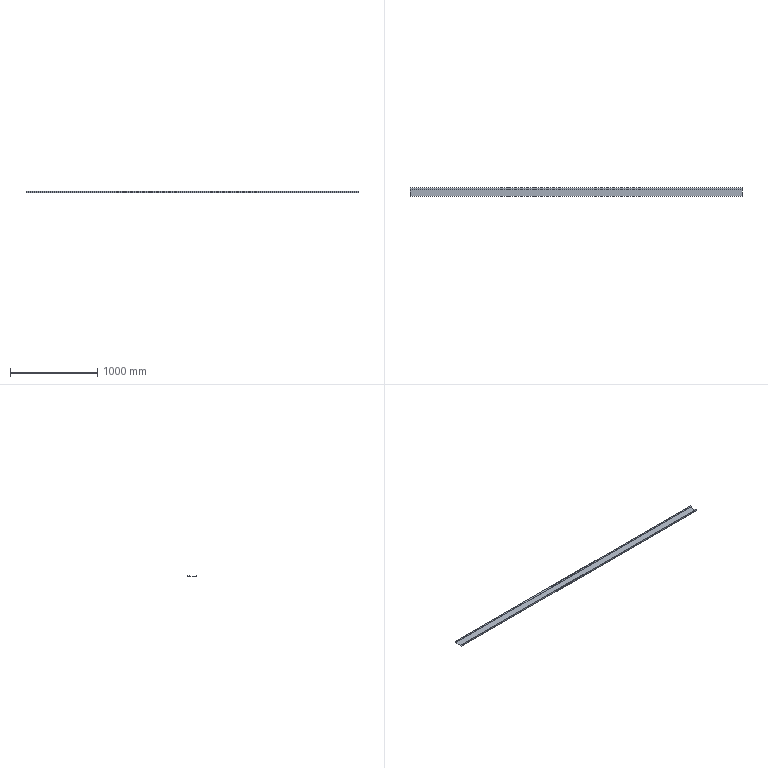Part | STEP file | 粉仓踢脚Plate 2 | 1 solid | 18 faces | box 3814 x 100 x 20 mm | volume 876724 mm3 | plane 12 | cylinder 6 | commonest cylinder face diameters 2 x3 5 x3
STEP:
#1=CARTESIAN_POINT('',(0.,0.,0.));
#2=DIRECTION('',(0.,0.,1.));
#3=DIRECTION('',(1.,0.,0.));
#4=AXIS2_PLACEMENT_3D('',#1,#2,#3);
#5=CARTESIAN_POINT('',(-1907.,1.5,2.5));
#6=VERTEX_POINT('',#5);
#7=CARTESIAN_POINT('',(-1907.,1.5,20.));
#8=VERTEX_POINT('',#7);
#9=CARTESIAN_POINT('',(-1907.,1.5,2.5));
#10=DIRECTION('',(0.,0.,1.));
#11=VECTOR('',#10,1.);
#12=LINE('',#9,#11);
#13=CARTESIAN_POINT('',(1907.,1.5,2.5));
#14=DIRECTION('',(0.,-1.,0.));
#15=DIRECTION('',(0.,0.,-1.));
#16=AXIS2_PLACEMENT_3D('',#13,#14,#15);
#17=PLANE('',#16);
#18=CARTESIAN_POINT('',(0.,-3814.));
#19=DIRECTION('',(-1.,0.));
#20=VECTOR('',#19,1.);
#21=LINE('',#18,#20);
#22=(GEOMETRIC_REPRESENTATION_CONTEXT(2)PARAMETRIC_REPRESENTATION_CONTEXT()REPRESENTATION_CONTEXT('',''));
#23=DEFINITIONAL_REPRESENTATION('',(#21),#22);
#24=PCURVE('',#17,#23);
#25=CARTESIAN_POINT('',(-1907.,2.5,2.5));
#26=DIRECTION('',(-1.,0.,0.));
#27=DIRECTION('',(0.,0.,1.));
#28=AXIS2_PLACEMENT_3D('',#25,#26,#27);
#29=PLANE('',#28);
#30=CARTESIAN_POINT('',(0.,-1.));
#31=DIRECTION('',(1.,0.));
#32=VECTOR('',#31,1.);
#33=LINE('',#30,#32);
#34=(GEOMETRIC_REPRESENTATION_CONTEXT(2)PARAMETRIC_REPRESENTATION_CONTEXT()REPRESENTATION_CONTEXT('',''));
#35=DEFINITIONAL_REPRESENTATION('',(#33),#34);
#36=PCURVE('',#29,#35);
#37=SURFACE_CURVE('',#12,(#24,#36),.PCURVE_S1.);
#38=EDGE_CURVE('',#6,#8,#37,.T.);
#39=ORIENTED_EDGE('',*,*,#38,.T.);
#40=CARTESIAN_POINT('',(1907.,1.5,20.));
#41=VERTEX_POINT('',#40);
#42=CARTESIAN_POINT('',(1907.,1.5,20.));
#43=DIRECTION('',(-1.,0.,0.));
#44=VECTOR('',#43,1.);
#45=LINE('',#42,#44);
#46=CARTESIAN_POINT('',(-17.5,0.));
#47=DIRECTION('',(0.,-1.));
#48=VECTOR('',#47,1.);
#49=LINE('',#46,#48);
#50=(GEOMETRIC_REPRESENTATION_CONTEXT(2)PARAMETRIC_REPRESENTATION_CONTEXT()REPRESENTATION_CONTEXT('',''));
#51=DEFINITIONAL_REPRESENTATION('',(#49),#50);
#52=PCURVE('',#17,#51);
#53=CARTESIAN_POINT('',(1907.,0.,20.));
#54=DIRECTION('',(0.,0.,1.));
#55=DIRECTION('',(1.,0.,0.));
#56=AXIS2_PLACEMENT_3D('',#53,#54,#55);
#57=PLANE('',#56);
#58=CARTESIAN_POINT('',(0.,1.5));
#59=DIRECTION('',(-1.,0.));
#60=VECTOR('',#59,1.);
#61=LINE('',#58,#60);
#62=(GEOMETRIC_REPRESENTATION_CONTEXT(2)PARAMETRIC_REPRESENTATION_CONTEXT()REPRESENTATION_CONTEXT('',''));
#63=DEFINITIONAL_REPRESENTATION('',(#61),#62);
#64=PCURVE('',#57,#63);
#65=SURFACE_CURVE('',#45,(#52,#64),.PCURVE_S1.);
#66=EDGE_CURVE('',#41,#8,#65,.T.);
#67=ORIENTED_EDGE('',*,*,#66,.F.);
#68=CARTESIAN_POINT('',(1907.,1.5,2.5));
#69=VERTEX_POINT('',#68);
#70=CARTESIAN_POINT('',(1907.,1.5,2.5));
#71=DIRECTION('',(0.,0.,1.));
#72=VECTOR('',#71,1.);
#73=LINE('',#70,#72);
#74=CARTESIAN_POINT('',(0.,0.));
#75=DIRECTION('',(-1.,0.));
#76=VECTOR('',#75,1.);
#77=LINE('',#74,#76);
#78=(GEOMETRIC_REPRESENTATION_CONTEXT(2)PARAMETRIC_REPRESENTATION_CONTEXT()REPRESENTATION_CONTEXT('',''));
#79=DEFINITIONAL_REPRESENTATION('',(#77),#78);
#80=PCURVE('',#17,#79);
#81=CARTESIAN_POINT('',(1907.,2.5,2.5));
#82=DIRECTION('',(-1.,0.,0.));
#83=DIRECTION('',(0.,0.,1.));
#84=AXIS2_PLACEMENT_3D('',#81,#82,#83);
#85=PLANE('',#84);
#86=CARTESIAN_POINT('',(0.,-1.));
#87=DIRECTION('',(1.,0.));
#88=VECTOR('',#87,1.);
#89=LINE('',#86,#88);
#90=(GEOMETRIC_REPRESENTATION_CONTEXT(2)PARAMETRIC_REPRESENTATION_CONTEXT()REPRESENTATION_CONTEXT('',''));
#91=DEFINITIONAL_REPRESENTATION('',(#89),#90);
#92=PCURVE('',#85,#91);
#93=SURFACE_CURVE('',#73,(#80,#92),.PCURVE_S1.);
#94=EDGE_CURVE('',#69,#41,#93,.T.);
#95=ORIENTED_EDGE('',*,*,#94,.F.);
#96=CARTESIAN_POINT('',(1907.,1.5,2.5));
#97=DIRECTION('',(-1.,0.,0.));
#98=VECTOR('',#97,1.);
#99=LINE('',#96,#98);
#100=CARTESIAN_POINT('',(0.,0.));
#101=DIRECTION('',(0.,-1.));
#102=VECTOR('',#101,1.);
#103=LINE('',#100,#102);
#104=(GEOMETRIC_REPRESENTATION_CONTEXT(2)PARAMETRIC_REPRESENTATION_CONTEXT()REPRESENTATION_CONTEXT('',''));
#105=DEFINITIONAL_REPRESENTATION('',(#103),#104);
#106=PCURVE('',#17,#105);
#107=CARTESIAN_POINT('',(1907.,2.5,2.5));
#108=DIRECTION('',(-1.,0.,0.));
#109=DIRECTION('',(0.,0.,1.));
#110=AXIS2_PLACEMENT_3D('',#107,#108,#109);
#111=CYLINDRICAL_SURFACE('',#110,1.);
#112=CARTESIAN_POINT('',(4.712,0.));
#113=DIRECTION('',(0.,1.));
#114=VECTOR('',#113,1.);
#115=LINE('',#112,#114);
#116=(GEOMETRIC_REPRESENTATION_CONTEXT(2)PARAMETRIC_REPRESENTATION_CONTEXT()REPRESENTATION_CONTEXT('',''));
#117=DEFINITIONAL_REPRESENTATION('',(#115),#116);
#118=PCURVE('',#111,#117);
#119=SURFACE_CURVE('',#99,(#106,#118),.PCURVE_S1.);
#120=EDGE_CURVE('',#69,#6,#119,.T.);
#121=ORIENTED_EDGE('',*,*,#120,.T.);
#122=EDGE_LOOP('',(#39,#67,#95,#121));
#123=FACE_BOUND('',#122,.T.);
#124=ADVANCED_FACE('',(#123),#17,.F.);
#125=CARTESIAN_POINT('',(-1907.,0.,20.));
#126=VERTEX_POINT('',#125);
#127=CARTESIAN_POINT('',(-1907.,0.,20.));
#128=DIRECTION('',(0.,1.,0.));
#129=VECTOR('',#128,1.);
#130=LINE('',#127,#129);
#131=CARTESIAN_POINT('',(-3814.,0.));
#132=DIRECTION('',(0.,1.));
#133=VECTOR('',#132,1.);
#134=LINE('',#131,#133);
#135=(GEOMETRIC_REPRESENTATION_CONTEXT(2)PARAMETRIC_REPRESENTATION_CONTEXT()REPRESENTATION_CONTEXT('',''));
#136=DEFINITIONAL_REPRESENTATION('',(#134),#135);
#137=PCURVE('',#57,#136);
#138=CARTESIAN_POINT('',(17.5,-2.5));
#139=DIRECTION('',(0.,1.));
#140=VECTOR('',#139,1.);
#141=LINE('',#138,#140);
#142=(GEOMETRIC_REPRESENTATION_CONTEXT(2)PARAMETRIC_REPRESENTATION_CONTEXT()REPRESENTATION_CONTEXT('',''));
#143=DEFINITIONAL_REPRESENTATION('',(#141),#142);
#144=PCURVE('',#29,#143);
#145=SURFACE_CURVE('',#130,(#137,#144),.PCURVE_S1.);
#146=EDGE_CURVE('',#126,#8,#145,.T.);
#147=ORIENTED_EDGE('',*,*,#146,.F.);
#148=CARTESIAN_POINT('',(1907.,0.,20.));
#149=VERTEX_POINT('',#148);
#150=CARTESIAN_POINT('',(1907.,0.,20.));
#151=DIRECTION('',(-1.,0.,0.));
#152=VECTOR('',#151,1.);
#153=LINE('',#150,#152);
#154=CARTESIAN_POINT('',(0.,0.));
#155=DIRECTION('',(-1.,0.));
#156=VECTOR('',#155,1.);
#157=LINE('',#154,#156);
#158=(GEOMETRIC_REPRESENTATION_CONTEXT(2)PARAMETRIC_REPRESENTATION_CONTEXT()REPRESENTATION_CONTEXT('',''));
#159=DEFINITIONAL_REPRESENTATION('',(#157),#158);
#160=PCURVE('',#57,#159);
#161=CARTESIAN_POINT('',(1907.,0.,2.5));
#162=DIRECTION('',(0.,-1.,0.));
#163=DIRECTION('',(0.,0.,-1.));
#164=AXIS2_PLACEMENT_3D('',#161,#162,#163);
#165=PLANE('',#164);
#166=CARTESIAN_POINT('',(-17.5,0.));
#167=DIRECTION('',(0.,-1.));
#168=VECTOR('',#167,1.);
#169=LINE('',#166,#168);
#170=(GEOMETRIC_REPRESENTATION_CONTEXT(2)PARAMETRIC_REPRESENTATION_CONTEXT()REPRESENTATION_CONTEXT('',''));
#171=DEFINITIONAL_REPRESENTATION('',(#169),#170);
#172=PCURVE('',#165,#171);
#173=SURFACE_CURVE('',#153,(#160,#172),.PCURVE_S1.);
#174=EDGE_CURVE('',#149,#126,#173,.T.);
#175=ORIENTED_EDGE('',*,*,#174,.F.);
#176=CARTESIAN_POINT('',(1907.,0.,20.));
#177=DIRECTION('',(0.,1.,0.));
#178=VECTOR('',#177,1.);
#179=LINE('',#176,#178);
#180=CARTESIAN_POINT('',(0.,0.));
#181=DIRECTION('',(0.,1.));
#182=VECTOR('',#181,1.);
#183=LINE('',#180,#182);
#184=(GEOMETRIC_REPRESENTATION_CONTEXT(2)PARAMETRIC_REPRESENTATION_CONTEXT()REPRESENTATION_CONTEXT('',''));
#185=DEFINITIONAL_REPRESENTATION('',(#183),#184);
#186=PCURVE('',#57,#185);
#187=CARTESIAN_POINT('',(17.5,-2.5));
#188=DIRECTION('',(0.,1.));
#189=VECTOR('',#188,1.);
#190=LINE('',#187,#189);
#191=(GEOMETRIC_REPRESENTATION_CONTEXT(2)PARAMETRIC_REPRESENTATION_CONTEXT()REPRESENTATION_CONTEXT('',''));
#192=DEFINITIONAL_REPRESENTATION('',(#190),#191);
#193=PCURVE('',#85,#192);
#194=SURFACE_CURVE('',#179,(#186,#193),.PCURVE_S1.);
#195=EDGE_CURVE('',#149,#41,#194,.T.);
#196=ORIENTED_EDGE('',*,*,#195,.T.);
#197=ORIENTED_EDGE('',*,*,#66,.T.);
#198=EDGE_LOOP('',(#147,#175,#196,#197));
#199=FACE_BOUND('',#198,.T.);
#200=ADVANCED_FACE('',(#199),#57,.T.);
#201=CARTESIAN_POINT('',(-1907.,0.,2.5));
#202=VERTEX_POINT('',#201);
#203=CARTESIAN_POINT('',(-1907.,0.,2.5));
#204=DIRECTION('',(0.,0.,1.));
#205=VECTOR('',#204,1.);
#206=LINE('',#203,#205);
#207=CARTESIAN_POINT('',(0.,-3814.));
#208=DIRECTION('',(-1.,0.));
#209=VECTOR('',#208,1.);
#210=LINE('',#207,#209);
#211=(GEOMETRIC_REPRESENTATION_CONTEXT(2)PARAMETRIC_REPRESENTATION_CONTEXT()REPRESENTATION_CONTEXT('',''));
#212=DEFINITIONAL_REPRESENTATION('',(#210),#211);
#213=PCURVE('',#165,#212);
#214=CARTESIAN_POINT('',(0.,-2.5));
#215=DIRECTION('',(1.,0.));
#216=VECTOR('',#215,1.);
#217=LINE('',#214,#216);
#218=(GEOMETRIC_REPRESENTATION_CONTEXT(2)PARAMETRIC_REPRESENTATION_CONTEXT()REPRESENTATION_CONTEXT('',''));
#219=DEFINITIONAL_REPRESENTATION('',(#217),#218);
#220=PCURVE('',#29,#219);
#221=SURFACE_CURVE('',#206,(#213,#220),.PCURVE_S1.);
#222=EDGE_CURVE('',#202,#126,#221,.T.);
#223=ORIENTED_EDGE('',*,*,#222,.F.);
#224=CARTESIAN_POINT('',(1907.,0.,2.5));
#225=VERTEX_POINT('',#224);
#226=CARTESIAN_POINT('',(1907.,0.,2.5));
#227=DIRECTION('',(-1.,0.,0.));
#228=VECTOR('',#227,1.);
#229=LINE('',#226,#228);
#230=CARTESIAN_POINT('',(0.,0.));
#231=DIRECTION('',(0.,-1.));
#232=VECTOR('',#231,1.);
#233=LINE('',#230,#232);
#234=(GEOMETRIC_REPRESENTATION_CONTEXT(2)PARAMETRIC_REPRESENTATION_CONTEXT()REPRESENTATION_CONTEXT('',''));
#235=DEFINITIONAL_REPRESENTATION('',(#233),#234);
#236=PCURVE('',#165,#235);
#237=CARTESIAN_POINT('',(1907.,2.5,2.5));
#238=DIRECTION('',(-1.,0.,0.));
#239=DIRECTION('',(0.,0.,1.));
#240=AXIS2_PLACEMENT_3D('',#237,#238,#239);
#241=CYLINDRICAL_SURFACE('',#240,2.5);
#242=CARTESIAN_POINT('',(4.712,0.));
#243=DIRECTION('',(0.,1.));
#244=VECTOR('',#243,1.);
#245=LINE('',#242,#244);
#246=(GEOMETRIC_REPRESENTATION_CONTEXT(2)PARAMETRIC_REPRESENTATION_CONTEXT()REPRESENTATION_CONTEXT('',''));
#247=DEFINITIONAL_REPRESENTATION('',(#245),#246);
#248=PCURVE('',#241,#247);
#249=SURFACE_CURVE('',#229,(#236,#248),.PCURVE_S1.);
#250=EDGE_CURVE('',#225,#202,#249,.T.);
#251=ORIENTED_EDGE('',*,*,#250,.F.);
#252=CARTESIAN_POINT('',(1907.,0.,2.5));
#253=DIRECTION('',(0.,0.,1.));
#254=VECTOR('',#253,1.);
#255=LINE('',#252,#254);
#256=CARTESIAN_POINT('',(0.,0.));
#257=DIRECTION('',(-1.,0.));
#258=VECTOR('',#257,1.);
#259=LINE('',#256,#258);
#260=(GEOMETRIC_REPRESENTATION_CONTEXT(2)PARAMETRIC_REPRESENTATION_CONTEXT()REPRESENTATION_CONTEXT('',''));
#261=DEFINITIONAL_REPRESENTATION('',(#259),#260);
#262=PCURVE('',#165,#261);
#263=CARTESIAN_POINT('',(0.,-2.5));
#264=DIRECTION('',(1.,0.));
#265=VECTOR('',#264,1.);
#266=LINE('',#263,#265);
#267=(GEOMETRIC_REPRESENTATION_CONTEXT(2)PARAMETRIC_REPRESENTATION_CONTEXT()REPRESENTATION_CONTEXT('',''));
#268=DEFINITIONAL_REPRESENTATION('',(#266),#267);
#269=PCURVE('',#85,#268);
#270=SURFACE_CURVE('',#255,(#262,#269),.PCURVE_S1.);
#271=EDGE_CURVE('',#225,#149,#270,.T.);
#272=ORIENTED_EDGE('',*,*,#271,.T.);
#273=ORIENTED_EDGE('',*,*,#174,.T.);
#274=EDGE_LOOP('',(#223,#251,#272,#273));
#275=FACE_BOUND('',#274,.T.);
#276=ADVANCED_FACE('',(#275),#165,.T.);
#277=CARTESIAN_POINT('',(-1907.,2.5,0.));
#278=VERTEX_POINT('',#277);
#279=CARTESIAN_POINT('',(-1907.,2.5,2.5));
#280=DIRECTION('',(-1.,0.,0.));
#281=DIRECTION('',(0.,0.,1.));
#282=AXIS2_PLACEMENT_3D('',#279,#280,#281);
#283=CIRCLE('',#282,2.5);
#284=CARTESIAN_POINT('',(0.,3814.));
#285=DIRECTION('',(1.,0.));
#286=VECTOR('',#285,1.);
#287=LINE('',#284,#286);
#288=(GEOMETRIC_REPRESENTATION_CONTEXT(2)PARAMETRIC_REPRESENTATION_CONTEXT()REPRESENTATION_CONTEXT('',''));
#289=DEFINITIONAL_REPRESENTATION('',(#287),#288);
#290=PCURVE('',#241,#289);
#291=CARTESIAN_POINT('',(0.,0.));
#292=DIRECTION('',(1.,0.));
#293=AXIS2_PLACEMENT_2D('',#291,#292);
#294=CIRCLE('',#293,2.5);
#295=(GEOMETRIC_REPRESENTATION_CONTEXT(2)PARAMETRIC_REPRESENTATION_CONTEXT()REPRESENTATION_CONTEXT('',''));
#296=DEFINITIONAL_REPRESENTATION('',(#294),#295);
#297=PCURVE('',#29,#296);
#298=SURFACE_CURVE('',#283,(#290,#297),.PCURVE_S1.);
#299=EDGE_CURVE('',#278,#202,#298,.T.);
#300=ORIENTED_EDGE('',*,*,#299,.F.);
#301=CARTESIAN_POINT('',(1907.,2.5,0.));
#302=VERTEX_POINT('',#301);
#303=CARTESIAN_POINT('',(1907.,2.5,0.));
#304=DIRECTION('',(-1.,0.,0.));
#305=VECTOR('',#304,1.);
#306=LINE('',#303,#305);
#307=CARTESIAN_POINT('',(3.142,0.));
#308=DIRECTION('',(0.,1.));
#309=VECTOR('',#308,1.);
#310=LINE('',#307,#309);
#311=(GEOMETRIC_REPRESENTATION_CONTEXT(2)PARAMETRIC_REPRESENTATION_CONTEXT()REPRESENTATION_CONTEXT('',''));
#312=DEFINITIONAL_REPRESENTATION('',(#310),#311);
#313=PCURVE('',#241,#312);
#314=CARTESIAN_POINT('',(1907.,2.5,0.));
#315=DIRECTION('',(0.,0.,-1.));
#316=DIRECTION('',(-1.,0.,0.));
#317=AXIS2_PLACEMENT_3D('',#314,#315,#316);
#318=PLANE('',#317);
#319=CARTESIAN_POINT('',(0.,0.));
#320=DIRECTION('',(1.,0.));
#321=VECTOR('',#320,1.);
#322=LINE('',#319,#321);
#323=(GEOMETRIC_REPRESENTATION_CONTEXT(2)PARAMETRIC_REPRESENTATION_CONTEXT()REPRESENTATION_CONTEXT('',''));
#324=DEFINITIONAL_REPRESENTATION('',(#322),#323);
#325=PCURVE('',#318,#324);
#326=SURFACE_CURVE('',#306,(#313,#325),.PCURVE_S1.);
#327=EDGE_CURVE('',#302,#278,#326,.T.);
#328=ORIENTED_EDGE('',*,*,#327,.F.);
#329=CARTESIAN_POINT('',(1907.,2.5,2.5));
#330=DIRECTION('',(-1.,0.,0.));
#331=DIRECTION('',(0.,0.,1.));
#332=AXIS2_PLACEMENT_3D('',#329,#330,#331);
#333=CIRCLE('',#332,2.5);
#334=CARTESIAN_POINT('',(0.,0.));
#335=DIRECTION('',(1.,0.));
#336=VECTOR('',#335,1.);
#337=LINE('',#334,#336);
#338=(GEOMETRIC_REPRESENTATION_CONTEXT(2)PARAMETRIC_REPRESENTATION_CONTEXT()REPRESENTATION_CONTEXT('',''));
#339=DEFINITIONAL_REPRESENTATION('',(#337),#338);
#340=PCURVE('',#241,#339);
#341=CARTESIAN_POINT('',(0.,0.));
#342=DIRECTION('',(1.,0.));
#343=AXIS2_PLACEMENT_2D('',#341,#342);
#344=CIRCLE('',#343,2.5);
#345=(GEOMETRIC_REPRESENTATION_CONTEXT(2)PARAMETRIC_REPRESENTATION_CONTEXT()REPRESENTATION_CONTEXT('',''));
#346=DEFINITIONAL_REPRESENTATION('',(#344),#345);
#347=PCURVE('',#85,#346);
#348=SURFACE_CURVE('',#333,(#340,#347),.PCURVE_S1.);
#349=EDGE_CURVE('',#302,#225,#348,.T.);
#350=ORIENTED_EDGE('',*,*,#349,.T.);
#351=ORIENTED_EDGE('',*,*,#250,.T.);
#352=EDGE_LOOP('',(#300,#328,#350,#351));
#353=FACE_BOUND('',#352,.T.);
#354=ADVANCED_FACE('',(#353),#241,.T.);
#355=CARTESIAN_POINT('',(-1907.,97.5,0.));
#356=VERTEX_POINT('',#355);
#357=CARTESIAN_POINT('',(-1907.,2.5,0.));
#358=DIRECTION('',(0.,-1.,0.));
#359=VECTOR('',#358,1.);
#360=LINE('',#357,#359);
#361=CARTESIAN_POINT('',(3814.,0.));
#362=DIRECTION('',(0.,-1.));
#363=VECTOR('',#362,1.);
#364=LINE('',#361,#363);
#365=(GEOMETRIC_REPRESENTATION_CONTEXT(2)PARAMETRIC_REPRESENTATION_CONTEXT()REPRESENTATION_CONTEXT('',''));
#366=DEFINITIONAL_REPRESENTATION('',(#364),#365);
#367=PCURVE('',#318,#366);
#368=CARTESIAN_POINT('',(-2.5,0.));
#369=DIRECTION('',(0.,-1.));
#370=VECTOR('',#369,1.);
#371=LINE('',#368,#370);
#372=(GEOMETRIC_REPRESENTATION_CONTEXT(2)PARAMETRIC_REPRESENTATION_CONTEXT()REPRESENTATION_CONTEXT('',''));
#373=DEFINITIONAL_REPRESENTATION('',(#371),#372);
#374=PCURVE('',#29,#373);
#375=SURFACE_CURVE('',#360,(#367,#374),.PCURVE_S1.);
#376=EDGE_CURVE('',#356,#278,#375,.T.);
#377=ORIENTED_EDGE('',*,*,#376,.F.);
#378=CARTESIAN_POINT('',(1907.,97.5,0.));
#379=VERTEX_POINT('',#378);
#380=CARTESIAN_POINT('',(1907.,97.5,0.));
#381=DIRECTION('',(-1.,0.,0.));
#382=VECTOR('',#381,1.);
#383=LINE('',#380,#382);
#384=CARTESIAN_POINT('',(0.,95.));
#385=DIRECTION('',(1.,0.));
#386=VECTOR('',#385,1.);
#387=LINE('',#384,#386);
#388=(GEOMETRIC_REPRESENTATION_CONTEXT(2)PARAMETRIC_REPRESENTATION_CONTEXT()REPRESENTATION_CONTEXT('',''));
#389=DEFINITIONAL_REPRESENTATION('',(#387),#388);
#390=PCURVE('',#318,#389);
#391=CARTESIAN_POINT('',(1907.,97.5,2.5));
#392=DIRECTION('',(-1.,0.,0.));
#393=DIRECTION('',(0.,0.,1.));
#394=AXIS2_PLACEMENT_3D('',#391,#392,#393);
#395=CYLINDRICAL_SURFACE('',#394,2.5);
#396=CARTESIAN_POINT('',(3.142,0.));
#397=DIRECTION('',(0.,1.));
#398=VECTOR('',#397,1.);
#399=LINE('',#396,#398);
#400=(GEOMETRIC_REPRESENTATION_CONTEXT(2)PARAMETRIC_REPRESENTATION_CONTEXT()REPRESENTATION_CONTEXT('',''));
#401=DEFINITIONAL_REPRESENTATION('',(#399),#400);
#402=PCURVE('',#395,#401);
#403=SURFACE_CURVE('',#383,(#390,#402),.PCURVE_S1.);
#404=EDGE_CURVE('',#379,#356,#403,.T.);
#405=ORIENTED_EDGE('',*,*,#404,.F.);
#406=CARTESIAN_POINT('',(1907.,2.5,0.));
#407=DIRECTION('',(0.,-1.,0.));
#408=VECTOR('',#407,1.);
#409=LINE('',#406,#408);
#410=CARTESIAN_POINT('',(0.,0.));
#411=DIRECTION('',(0.,-1.));
#412=VECTOR('',#411,1.);
#413=LINE('',#410,#412);
#414=(GEOMETRIC_REPRESENTATION_CONTEXT(2)PARAMETRIC_REPRESENTATION_CONTEXT()REPRESENTATION_CONTEXT('',''));
#415=DEFINITIONAL_REPRESENTATION('',(#413),#414);
#416=PCURVE('',#318,#415);
#417=CARTESIAN_POINT('',(-2.5,0.));
#418=DIRECTION('',(0.,-1.));
#419=VECTOR('',#418,1.);
#420=LINE('',#417,#419);
#421=(GEOMETRIC_REPRESENTATION_CONTEXT(2)PARAMETRIC_REPRESENTATION_CONTEXT()REPRESENTATION_CONTEXT('',''));
#422=DEFINITIONAL_REPRESENTATION('',(#420),#421);
#423=PCURVE('',#85,#422);
#424=SURFACE_CURVE('',#409,(#416,#423),.PCURVE_S1.);
#425=EDGE_CURVE('',#379,#302,#424,.T.);
#426=ORIENTED_EDGE('',*,*,#425,.T.);
#427=ORIENTED_EDGE('',*,*,#327,.T.);
#428=EDGE_LOOP('',(#377,#405,#426,#427));
#429=FACE_BOUND('',#428,.T.);
#430=ADVANCED_FACE('',(#429),#318,.T.);
#431=CARTESIAN_POINT('',(-1907.,100.,2.5));
#432=VERTEX_POINT('',#431);
#433=CARTESIAN_POINT('',(-1907.,97.5,2.5));
#434=DIRECTION('',(-1.,0.,0.));
#435=DIRECTION('',(0.,0.,-1.));
#436=AXIS2_PLACEMENT_3D('',#433,#434,#435);
#437=CIRCLE('',#436,2.5);
#438=CARTESIAN_POINT('',(-3.142,3814.));
#439=DIRECTION('',(1.,0.));
#440=VECTOR('',#439,1.);
#441=LINE('',#438,#440);
#442=(GEOMETRIC_REPRESENTATION_CONTEXT(2)PARAMETRIC_REPRESENTATION_CONTEXT()REPRESENTATION_CONTEXT('',''));
#443=DEFINITIONAL_REPRESENTATION('',(#441),#442);
#444=PCURVE('',#395,#443);
#445=CARTESIAN_POINT('',(0.,95.));
#446=DIRECTION('',(-1.,0.));
#447=AXIS2_PLACEMENT_2D('',#445,#446);
#448=CIRCLE('',#447,2.5);
#449=(GEOMETRIC_REPRESENTATION_CONTEXT(2)PARAMETRIC_REPRESENTATION_CONTEXT()REPRESENTATION_CONTEXT('',''));
#450=DEFINITIONAL_REPRESENTATION('',(#448),#449);
#451=PCURVE('',#29,#450);
#452=SURFACE_CURVE('',#437,(#444,#451),.PCURVE_S1.);
#453=EDGE_CURVE('',#432,#356,#452,.T.);
#454=ORIENTED_EDGE('',*,*,#453,.F.);
#455=CARTESIAN_POINT('',(1907.,100.,2.5));
#456=VERTEX_POINT('',#455);
#457=CARTESIAN_POINT('',(1907.,100.,2.5));
#458=DIRECTION('',(-1.,0.,0.));
#459=VECTOR('',#458,1.);
#460=LINE('',#457,#459);
#461=CARTESIAN_POINT('',(1.571,0.));
#462=DIRECTION('',(0.,1.));
#463=VECTOR('',#462,1.);
#464=LINE('',#461,#463);
#465=(GEOMETRIC_REPRESENTATION_CONTEXT(2)PARAMETRIC_REPRESENTATION_CONTEXT()REPRESENTATION_CONTEXT('',''));
#466=DEFINITIONAL_REPRESENTATION('',(#464),#465);
#467=PCURVE('',#395,#466);
#468=CARTESIAN_POINT('',(1907.,100.,2.5));
#469=DIRECTION('',(0.,1.,0.));
#470=DIRECTION('',(0.,0.,1.));
#471=AXIS2_PLACEMENT_3D('',#468,#469,#470);
#472=PLANE('',#471);
#473=CARTESIAN_POINT('',(0.,0.));
#474=DIRECTION('',(0.,-1.));
#475=VECTOR('',#474,1.);
#476=LINE('',#473,#475);
#477=(GEOMETRIC_REPRESENTATION_CONTEXT(2)PARAMETRIC_REPRESENTATION_CONTEXT()REPRESENTATION_CONTEXT('',''));
#478=DEFINITIONAL_REPRESENTATION('',(#476),#477);
#479=PCURVE('',#472,#478);
#480=SURFACE_CURVE('',#460,(#467,#479),.PCURVE_S1.);
#481=EDGE_CURVE('',#456,#432,#480,.T.);
#482=ORIENTED_EDGE('',*,*,#481,.F.);
#483=CARTESIAN_POINT('',(1907.,97.5,2.5));
#484=DIRECTION('',(-1.,0.,0.));
#485=DIRECTION('',(0.,0.,-1.));
#486=AXIS2_PLACEMENT_3D('',#483,#484,#485);
#487=CIRCLE('',#486,2.5);
#488=CARTESIAN_POINT('',(-3.142,0.));
#489=DIRECTION('',(1.,0.));
#490=VECTOR('',#489,1.);
#491=LINE('',#488,#490);
#492=(GEOMETRIC_REPRESENTATION_CONTEXT(2)PARAMETRIC_REPRESENTATION_CONTEXT()REPRESENTATION_CONTEXT('',''));
#493=DEFINITIONAL_REPRESENTATION('',(#491),#492);
#494=PCURVE('',#395,#493);
#495=CARTESIAN_POINT('',(0.,95.));
#496=DIRECTION('',(-1.,0.));
#497=AXIS2_PLACEMENT_2D('',#495,#496);
#498=CIRCLE('',#497,2.5);
#499=(GEOMETRIC_REPRESENTATION_CONTEXT(2)PARAMETRIC_REPRESENTATION_CONTEXT()REPRESENTATION_CONTEXT('',''));
#500=DEFINITIONAL_REPRESENTATION('',(#498),#499);
#501=PCURVE('',#85,#500);
#502=SURFACE_CURVE('',#487,(#494,#501),.PCURVE_S1.);
#503=EDGE_CURVE('',#456,#379,#502,.T.);
#504=ORIENTED_EDGE('',*,*,#503,.T.);
#505=ORIENTED_EDGE('',*,*,#404,.T.);
#506=EDGE_LOOP('',(#454,#482,#504,#505));
#507=FACE_BOUND('',#506,.T.);
#508=ADVANCED_FACE('',(#507),#395,.T.);
#509=CARTESIAN_POINT('',(-1907.,100.,17.5));
#510=VERTEX_POINT('',#509);
#511=CARTESIAN_POINT('',(-1907.,100.,2.5));
#512=DIRECTION('',(0.,0.,-1.));
#513=VECTOR('',#512,1.);
#514=LINE('',#511,#513);
#515=CARTESIAN_POINT('',(0.,-3814.));
#516=DIRECTION('',(-1.,0.));
#517=VECTOR('',#516,1.);
#518=LINE('',#515,#517);
#519=(GEOMETRIC_REPRESENTATION_CONTEXT(2)PARAMETRIC_REPRESENTATION_CONTEXT()REPRESENTATION_CONTEXT('',''));
#520=DEFINITIONAL_REPRESENTATION('',(#518),#519);
#521=PCURVE('',#472,#520);
#522=CARTESIAN_POINT('',(0.,97.5));
#523=DIRECTION('',(-1.,0.));
#524=VECTOR('',#523,1.);
#525=LINE('',#522,#524);
#526=(GEOMETRIC_REPRESENTATION_CONTEXT(2)PARAMETRIC_REPRESENTATION_CONTEXT()REPRESENTATION_CONTEXT('',''));
#527=DEFINITIONAL_REPRESENTATION('',(#525),#526);
#528=PCURVE('',#29,#527);
#529=SURFACE_CURVE('',#514,(#521,#528),.PCURVE_S1.);
#530=EDGE_CURVE('',#510,#432,#529,.T.);
#531=ORIENTED_EDGE('',*,*,#530,.F.);
#532=CARTESIAN_POINT('',(1907.,100.,17.5));
#533=VERTEX_POINT('',#532);
#534=CARTESIAN_POINT('',(1907.,100.,17.5));
#535=DIRECTION('',(-1.,0.,0.));
#536=VECTOR('',#535,1.);
#537=LINE('',#534,#536);
#538=CARTESIAN_POINT('',(15.,0.));
#539=DIRECTION('',(0.,-1.));
#540=VECTOR('',#539,1.);
#541=LINE('',#538,#540);
#542=(GEOMETRIC_REPRESENTATION_CONTEXT(2)PARAMETRIC_REPRESENTATION_CONTEXT()REPRESENTATION_CONTEXT('',''));
#543=DEFINITIONAL_REPRESENTATION('',(#541),#542);
#544=PCURVE('',#472,#543);
#545=CARTESIAN_POINT('',(1907.,97.5,17.5));
#546=DIRECTION('',(-1.,0.,0.));
#547=DIRECTION('',(0.,0.,1.));
#548=AXIS2_PLACEMENT_3D('',#545,#546,#547);
#549=CYLINDRICAL_SURFACE('',#548,2.5);
#550=CARTESIAN_POINT('',(1.571,0.));
#551=DIRECTION('',(0.,1.));
#552=VECTOR('',#551,1.);
#553=LINE('',#550,#552);
#554=(GEOMETRIC_REPRESENTATION_CONTEXT(2)PARAMETRIC_REPRESENTATION_CONTEXT()REPRESENTATION_CONTEXT('',''));
#555=DEFINITIONAL_REPRESENTATION('',(#553),#554);
#556=PCURVE('',#549,#555);
#557=SURFACE_CURVE('',#537,(#544,#556),.PCURVE_S1.);
#558=EDGE_CURVE('',#533,#510,#557,.T.);
#559=ORIENTED_EDGE('',*,*,#558,.F.);
#560=CARTESIAN_POINT('',(1907.,100.,2.5));
#561=DIRECTION('',(0.,0.,-1.));
#562=VECTOR('',#561,1.);
#563=LINE('',#560,#562);
#564=CARTESIAN_POINT('',(0.,0.));
#565=DIRECTION('',(-1.,0.));
#566=VECTOR('',#565,1.);
#567=LINE('',#564,#566);
#568=(GEOMETRIC_REPRESENTATION_CONTEXT(2)PARAMETRIC_REPRESENTATION_CONTEXT()REPRESENTATION_CONTEXT('',''));
#569=DEFINITIONAL_REPRESENTATION('',(#567),#568);
#570=PCURVE('',#472,#569);
#571=CARTESIAN_POINT('',(0.,97.5));
#572=DIRECTION('',(-1.,0.));
#573=VECTOR('',#572,1.);
#574=LINE('',#571,#573);
#575=(GEOMETRIC_REPRESENTATION_CONTEXT(2)PARAMETRIC_REPRESENTATION_CONTEXT()REPRESENTATION_CONTEXT('',''));
#576=DEFINITIONAL_REPRESENTATION('',(#574),#575);
#577=PCURVE('',#85,#576);
#578=SURFACE_CURVE('',#563,(#570,#577),.PCURVE_S1.);
#579=EDGE_CURVE('',#533,#456,#578,.T.);
#580=ORIENTED_EDGE('',*,*,#579,.T.);
#581=ORIENTED_EDGE('',*,*,#481,.T.);
#582=EDGE_LOOP('',(#531,#559,#580,#581));
#583=FACE_BOUND('',#582,.T.);
#584=ADVANCED_FACE('',(#583),#472,.T.);
#585=CARTESIAN_POINT('',(-1907.,97.5,20.));
#586=VERTEX_POINT('',#585);
#587=CARTESIAN_POINT('',(-1907.,97.5,17.5));
#588=DIRECTION('',(-1.,0.,0.));
#589=DIRECTION('',(0.,0.,-1.));
#590=AXIS2_PLACEMENT_3D('',#587,#588,#589);
#591=CIRCLE('',#590,2.5);
#592=CARTESIAN_POINT('',(-3.142,3814.));
#593=DIRECTION('',(1.,0.));
#594=VECTOR('',#593,1.);
#595=LINE('',#592,#594);
#596=(GEOMETRIC_REPRESENTATION_CONTEXT(2)PARAMETRIC_REPRESENTATION_CONTEXT()REPRESENTATION_CONTEXT('',''));
#597=DEFINITIONAL_REPRESENTATION('',(#595),#596);
#598=PCURVE('',#549,#597);
#599=CARTESIAN_POINT('',(15.,95.));
#600=DIRECTION('',(-1.,0.));
#601=AXIS2_PLACEMENT_2D('',#599,#600);
#602=CIRCLE('',#601,2.5);
#603=(GEOMETRIC_REPRESENTATION_CONTEXT(2)PARAMETRIC_REPRESENTATION_CONTEXT()REPRESENTATION_CONTEXT('',''));
#604=DEFINITIONAL_REPRESENTATION('',(#602),#603);
#605=PCURVE('',#29,#604);
#606=SURFACE_CURVE('',#591,(#598,#605),.PCURVE_S1.);
#607=EDGE_CURVE('',#586,#510,#606,.T.);
#608=ORIENTED_EDGE('',*,*,#607,.F.);
#609=CARTESIAN_POINT('',(1907.,97.5,20.));
#610=VERTEX_POINT('',#609);
#611=CARTESIAN_POINT('',(1907.,97.5,20.));
#612=DIRECTION('',(-1.,0.,0.));
#613=VECTOR('',#612,1.);
#614=LINE('',#611,#613);
#615=CARTESIAN_POINT('',(0.,0.));
#616=DIRECTION('',(0.,1.));
#617=VECTOR('',#616,1.);
#618=LINE('',#615,#617);
#619=(GEOMETRIC_REPRESENTATION_CONTEXT(2)PARAMETRIC_REPRESENTATION_CONTEXT()REPRESENTATION_CONTEXT('',''));
#620=DEFINITIONAL_REPRESENTATION('',(#618),#619);
#621=PCURVE('',#549,#620);
#622=CARTESIAN_POINT('',(1907.,97.5,20.));
#623=DIRECTION('',(0.,0.,1.));
#624=DIRECTION('',(1.,0.,0.));
#625=AXIS2_PLACEMENT_3D('',#622,#623,#624);
#626=PLANE('',#625);
#627=CARTESIAN_POINT('',(0.,0.));
#628=DIRECTION('',(-1.,0.));
#629=VECTOR('',#628,1.);
#630=LINE('',#627,#629);
#631=(GEOMETRIC_REPRESENTATION_CONTEXT(2)PARAMETRIC_REPRESENTATION_CONTEXT()REPRESENTATION_CONTEXT('',''));
#632=DEFINITIONAL_REPRESENTATION('',(#630),#631);
#633=PCURVE('',#626,#632);
#634=SURFACE_CURVE('',#614,(#621,#633),.PCURVE_S1.);
#635=EDGE_CURVE('',#610,#586,#634,.T.);
#636=ORIENTED_EDGE('',*,*,#635,.F.);
#637=CARTESIAN_POINT('',(1907.,97.5,17.5));
#638=DIRECTION('',(-1.,0.,0.));
#639=DIRECTION('',(0.,0.,-1.));
#640=AXIS2_PLACEMENT_3D('',#637,#638,#639);
#641=CIRCLE('',#640,2.5);
#642=CARTESIAN_POINT('',(-3.142,0.));
#643=DIRECTION('',(1.,0.));
#644=VECTOR('',#643,1.);
#645=LINE('',#642,#644);
#646=(GEOMETRIC_REPRESENTATION_CONTEXT(2)PARAMETRIC_REPRESENTATION_CONTEXT()REPRESENTATION_CONTEXT('',''));
#647=DEFINITIONAL_REPRESENTATION('',(#645),#646);
#648=PCURVE('',#549,#647);
#649=CARTESIAN_POINT('',(15.,95.));
#650=DIRECTION('',(-1.,0.));
#651=AXIS2_PLACEMENT_2D('',#649,#650);
#652=CIRCLE('',#651,2.5);
#653=(GEOMETRIC_REPRESENTATION_CONTEXT(2)PARAMETRIC_REPRESENTATION_CONTEXT()REPRESENTATION_CONTEXT('',''));
#654=DEFINITIONAL_REPRESENTATION('',(#652),#653);
#655=PCURVE('',#85,#654);
#656=SURFACE_CURVE('',#641,(#648,#655),.PCURVE_S1.);
#657=EDGE_CURVE('',#610,#533,#656,.T.);
#658=ORIENTED_EDGE('',*,*,#657,.T.);
#659=ORIENTED_EDGE('',*,*,#558,.T.);
#660=EDGE_LOOP('',(#608,#636,#658,#659));
#661=FACE_BOUND('',#660,.T.);
#662=ADVANCED_FACE('',(#661),#549,.T.);
#663=CARTESIAN_POINT('',(-1907.,80.,20.));
#664=VERTEX_POINT('',#663);
#665=CARTESIAN_POINT('',(-1907.,97.5,20.));
#666=DIRECTION('',(0.,1.,0.));
#667=VECTOR('',#666,1.);
#668=LINE('',#665,#667);
#669=CARTESIAN_POINT('',(-3814.,0.));
#670=DIRECTION('',(0.,1.));
#671=VECTOR('',#670,1.);
#672=LINE('',#669,#671);
#673=(GEOMETRIC_REPRESENTATION_CONTEXT(2)PARAMETRIC_REPRESENTATION_CONTEXT()REPRESENTATION_CONTEXT('',''));
#674=DEFINITIONAL_REPRESENTATION('',(#672),#673);
#675=PCURVE('',#626,#674);
#676=CARTESIAN_POINT('',(17.5,95.));
#677=DIRECTION('',(0.,1.));
#678=VECTOR('',#677,1.);
#679=LINE('',#676,#678);
#680=(GEOMETRIC_REPRESENTATION_CONTEXT(2)PARAMETRIC_REPRESENTATION_CONTEXT()REPRESENTATION_CONTEXT('',''));
#681=DEFINITIONAL_REPRESENTATION('',(#679),#680);
#682=PCURVE('',#29,#681);
#683=SURFACE_CURVE('',#668,(#675,#682),.PCURVE_S1.);
#684=EDGE_CURVE('',#664,#586,#683,.T.);
#685=ORIENTED_EDGE('',*,*,#684,.F.);
#686=CARTESIAN_POINT('',(1907.,80.,20.));
#687=VERTEX_POINT('',#686);
#688=CARTESIAN_POINT('',(1907.,80.,20.));
#689=DIRECTION('',(-1.,0.,0.));
#690=VECTOR('',#689,1.);
#691=LINE('',#688,#690);
#692=CARTESIAN_POINT('',(0.,-17.5));
#693=DIRECTION('',(-1.,0.));
#694=VECTOR('',#693,1.);
#695=LINE('',#692,#694);
#696=(GEOMETRIC_REPRESENTATION_CONTEXT(2)PARAMETRIC_REPRESENTATION_CONTEXT()REPRESENTATION_CONTEXT('',''));
#697=DEFINITIONAL_REPRESENTATION('',(#695),#696);
#698=PCURVE('',#626,#697);
#699=CARTESIAN_POINT('',(1907.,80.,18.5));
#700=DIRECTION('',(0.,-1.,0.));
#701=DIRECTION('',(0.,0.,-1.));
#702=AXIS2_PLACEMENT_3D('',#699,#700,#701);
#703=PLANE('',#702);
#704=CARTESIAN_POINT('',(-1.5,0.));
#705=DIRECTION('',(0.,-1.));
#706=VECTOR('',#705,1.);
#707=LINE('',#704,#706);
#708=(GEOMETRIC_REPRESENTATION_CONTEXT(2)PARAMETRIC_REPRESENTATION_CONTEXT()REPRESENTATION_CONTEXT('',''));
#709=DEFINITIONAL_REPRESENTATION('',(#707),#708);
#710=PCURVE('',#703,#709);
#711=SURFACE_CURVE('',#691,(#698,#710),.PCURVE_S1.);
#712=EDGE_CURVE('',#687,#664,#711,.T.);
#713=ORIENTED_EDGE('',*,*,#712,.F.);
#714=CARTESIAN_POINT('',(1907.,97.5,20.));
#715=DIRECTION('',(0.,1.,0.));
#716=VECTOR('',#715,1.);
#717=LINE('',#714,#716);
#718=CARTESIAN_POINT('',(0.,0.));
#719=DIRECTION('',(0.,1.));
#720=VECTOR('',#719,1.);
#721=LINE('',#718,#720);
#722=(GEOMETRIC_REPRESENTATION_CONTEXT(2)PARAMETRIC_REPRESENTATION_CONTEXT()REPRESENTATION_CONTEXT('',''));
#723=DEFINITIONAL_REPRESENTATION('',(#721),#722);
#724=PCURVE('',#626,#723);
#725=CARTESIAN_POINT('',(17.5,95.));
#726=DIRECTION('',(0.,1.));
#727=VECTOR('',#726,1.);
#728=LINE('',#725,#727);
#729=(GEOMETRIC_REPRESENTATION_CONTEXT(2)PARAMETRIC_REPRESENTATION_CONTEXT()REPRESENTATION_CONTEXT('',''));
#730=DEFINITIONAL_REPRESENTATION('',(#728),#729);
#731=PCURVE('',#85,#730);
#732=SURFACE_CURVE('',#717,(#724,#731),.PCURVE_S1.);
#733=EDGE_CURVE('',#687,#610,#732,.T.);
#734=ORIENTED_EDGE('',*,*,#733,.T.);
#735=ORIENTED_EDGE('',*,*,#635,.T.);
#736=EDGE_LOOP('',(#685,#713,#734,#735));
#737=FACE_BOUND('',#736,.T.);
#738=ADVANCED_FACE('',(#737),#626,.T.);
#739=CARTESIAN_POINT('',(-1907.,80.,18.5));
#740=VERTEX_POINT('',#739);
#741=CARTESIAN_POINT('',(-1907.,80.,18.5));
#742=DIRECTION('',(0.,0.,1.));
#743=VECTOR('',#742,1.);
#744=LINE('',#741,#743);
#745=CARTESIAN_POINT('',(0.,-3814.));
#746=DIRECTION('',(-1.,0.));
#747=VECTOR('',#746,1.);
#748=LINE('',#745,#747);
#749=(GEOMETRIC_REPRESENTATION_CONTEXT(2)PARAMETRIC_REPRESENTATION_CONTEXT()REPRESENTATION_CONTEXT('',''));
#750=DEFINITIONAL_REPRESENTATION('',(#748),#749);
#751=PCURVE('',#703,#750);
#752=CARTESIAN_POINT('',(16.,77.5));
#753=DIRECTION('',(1.,0.));
#754=VECTOR('',#753,1.);
#755=LINE('',#752,#754);
#756=(GEOMETRIC_REPRESENTATION_CONTEXT(2)PARAMETRIC_REPRESENTATION_CONTEXT()REPRESENTATION_CONTEXT('',''));
#757=DEFINITIONAL_REPRESENTATION('',(#755),#756);
#758=PCURVE('',#29,#757);
#759=SURFACE_CURVE('',#744,(#751,#758),.PCURVE_S1.);
#760=EDGE_CURVE('',#740,#664,#759,.T.);
#761=ORIENTED_EDGE('',*,*,#760,.F.);
#762=CARTESIAN_POINT('',(1907.,80.,18.5));
#763=VERTEX_POINT('',#762);
#764=CARTESIAN_POINT('',(1907.,80.,18.5));
#765=DIRECTION('',(-1.,0.,0.));
#766=VECTOR('',#765,1.);
#767=LINE('',#764,#766);
#768=CARTESIAN_POINT('',(0.,0.));
#769=DIRECTION('',(0.,-1.));
#770=VECTOR('',#769,1.);
#771=LINE('',#768,#770);
#772=(GEOMETRIC_REPRESENTATION_CONTEXT(2)PARAMETRIC_REPRESENTATION_CONTEXT()REPRESENTATION_CONTEXT('',''));
#773=DEFINITIONAL_REPRESENTATION('',(#771),#772);
#774=PCURVE('',#703,#773);
#775=CARTESIAN_POINT('',(1907.,97.5,18.5));
#776=DIRECTION('',(0.,0.,1.));
#777=DIRECTION('',(1.,0.,0.));
#778=AXIS2_PLACEMENT_3D('',#775,#776,#777);
#779=PLANE('',#778);
#780=CARTESIAN_POINT('',(0.,-17.5));
#781=DIRECTION('',(-1.,0.));
#782=VECTOR('',#781,1.);
#783=LINE('',#780,#782);
#784=(GEOMETRIC_REPRESENTATION_CONTEXT(2)PARAMETRIC_REPRESENTATION_CONTEXT()REPRESENTATION_CONTEXT('',''));
#785=DEFINITIONAL_REPRESENTATION('',(#783),#784);
#786=PCURVE('',#779,#785);
#787=SURFACE_CURVE('',#767,(#774,#786),.PCURVE_S1.);
#788=EDGE_CURVE('',#763,#740,#787,.T.);
#789=ORIENTED_EDGE('',*,*,#788,.F.);
#790=CARTESIAN_POINT('',(1907.,80.,18.5));
#791=DIRECTION('',(0.,0.,1.));
#792=VECTOR('',#791,1.);
#793=LINE('',#790,#792);
#794=CARTESIAN_POINT('',(0.,0.));
#795=DIRECTION('',(-1.,0.));
#796=VECTOR('',#795,1.);
#797=LINE('',#794,#796);
#798=(GEOMETRIC_REPRESENTATION_CONTEXT(2)PARAMETRIC_REPRESENTATION_CONTEXT()REPRESENTATION_CONTEXT('',''));
#799=DEFINITIONAL_REPRESENTATION('',(#797),#798);
#800=PCURVE('',#703,#799);
#801=CARTESIAN_POINT('',(16.,77.5));
#802=DIRECTION('',(1.,0.));
#803=VECTOR('',#802,1.);
#804=LINE('',#801,#803);
#805=(GEOMETRIC_REPRESENTATION_CONTEXT(2)PARAMETRIC_REPRESENTATION_CONTEXT()REPRESENTATION_CONTEXT('',''));
#806=DEFINITIONAL_REPRESENTATION('',(#804),#805);
#807=PCURVE('',#85,#806);
#808=SURFACE_CURVE('',#793,(#800,#807),.PCURVE_S1.);
#809=EDGE_CURVE('',#763,#687,#808,.T.);
#810=ORIENTED_EDGE('',*,*,#809,.T.);
#811=ORIENTED_EDGE('',*,*,#712,.T.);
#812=EDGE_LOOP('',(#761,#789,#810,#811));
#813=FACE_BOUND('',#812,.T.);
#814=ADVANCED_FACE('',(#813),#703,.T.);
#815=CARTESIAN_POINT('',(-1907.,97.5,18.5));
#816=VERTEX_POINT('',#815);
#817=CARTESIAN_POINT('',(-1907.,97.5,18.5));
#818=DIRECTION('',(0.,1.,0.));
#819=VECTOR('',#818,1.);
#820=LINE('',#817,#819);
#821=CARTESIAN_POINT('',(-3814.,0.));
#822=DIRECTION('',(0.,1.));
#823=VECTOR('',#822,1.);
#824=LINE('',#821,#823);
#825=(GEOMETRIC_REPRESENTATION_CONTEXT(2)PARAMETRIC_REPRESENTATION_CONTEXT()REPRESENTATION_CONTEXT('',''));
#826=DEFINITIONAL_REPRESENTATION('',(#824),#825);
#827=PCURVE('',#779,#826);
#828=CARTESIAN_POINT('',(16.,95.));
#829=DIRECTION('',(0.,1.));
#830=VECTOR('',#829,1.);
#831=LINE('',#828,#830);
#832=(GEOMETRIC_REPRESENTATION_CONTEXT(2)PARAMETRIC_REPRESENTATION_CONTEXT()REPRESENTATION_CONTEXT('',''));
#833=DEFINITIONAL_REPRESENTATION('',(#831),#832);
#834=PCURVE('',#29,#833);
#835=SURFACE_CURVE('',#820,(#827,#834),.PCURVE_S1.);
#836=EDGE_CURVE('',#740,#816,#835,.T.);
#837=ORIENTED_EDGE('',*,*,#836,.T.);
#838=CARTESIAN_POINT('',(1907.,97.5,18.5));
#839=VERTEX_POINT('',#838);
#840=CARTESIAN_POINT('',(1907.,97.5,18.5));
#841=DIRECTION('',(-1.,0.,0.));
#842=VECTOR('',#841,1.);
#843=LINE('',#840,#842);
#844=CARTESIAN_POINT('',(0.,0.));
#845=DIRECTION('',(-1.,0.));
#846=VECTOR('',#845,1.);
#847=LINE('',#844,#846);
#848=(GEOMETRIC_REPRESENTATION_CONTEXT(2)PARAMETRIC_REPRESENTATION_CONTEXT()REPRESENTATION_CONTEXT('',''));
#849=DEFINITIONAL_REPRESENTATION('',(#847),#848);
#850=PCURVE('',#779,#849);
#851=CARTESIAN_POINT('',(1907.,97.5,17.5));
#852=DIRECTION('',(-1.,0.,0.));
#853=DIRECTION('',(0.,0.,1.));
#854=AXIS2_PLACEMENT_3D('',#851,#852,#853);
#855=CYLINDRICAL_SURFACE('',#854,1.);
#856=CARTESIAN_POINT('',(0.,0.));
#857=DIRECTION('',(0.,1.));
#858=VECTOR('',#857,1.);
#859=LINE('',#856,#858);
#860=(GEOMETRIC_REPRESENTATION_CONTEXT(2)PARAMETRIC_REPRESENTATION_CONTEXT()REPRESENTATION_CONTEXT('',''));
#861=DEFINITIONAL_REPRESENTATION('',(#859),#860);
#862=PCURVE('',#855,#861);
#863=SURFACE_CURVE('',#843,(#850,#862),.PCURVE_S1.);
#864=EDGE_CURVE('',#839,#816,#863,.T.);
#865=ORIENTED_EDGE('',*,*,#864,.F.);
#866=CARTESIAN_POINT('',(1907.,97.5,18.5));
#867=DIRECTION('',(0.,1.,0.));
#868=VECTOR('',#867,1.);
#869=LINE('',#866,#868);
#870=CARTESIAN_POINT('',(0.,0.));
#871=DIRECTION('',(0.,1.));
#872=VECTOR('',#871,1.);
#873=LINE('',#870,#872);
#874=(GEOMETRIC_REPRESENTATION_CONTEXT(2)PARAMETRIC_REPRESENTATION_CONTEXT()REPRESENTATION_CONTEXT('',''));
#875=DEFINITIONAL_REPRESENTATION('',(#873),#874);
#876=PCURVE('',#779,#875);
#877=CARTESIAN_POINT('',(16.,95.));
#878=DIRECTION('',(0.,1.));
#879=VECTOR('',#878,1.);
#880=LINE('',#877,#879);
#881=(GEOMETRIC_REPRESENTATION_CONTEXT(2)PARAMETRIC_REPRESENTATION_CONTEXT()REPRESENTATION_CONTEXT('',''));
#882=DEFINITIONAL_REPRESENTATION('',(#880),#881);
#883=PCURVE('',#85,#882);
#884=SURFACE_CURVE('',#869,(#876,#883),.PCURVE_S1.);
#885=EDGE_CURVE('',#763,#839,#884,.T.);
#886=ORIENTED_EDGE('',*,*,#885,.F.);
#887=ORIENTED_EDGE('',*,*,#788,.T.);
#888=EDGE_LOOP('',(#837,#865,#886,#887));
#889=FACE_BOUND('',#888,.T.);
#890=ADVANCED_FACE('',(#889),#779,.F.);
#891=ORIENTED_EDGE('',*,*,#864,.F.);
#892=CARTESIAN_POINT('',(1907.,98.5,17.5));
#893=VERTEX_POINT('',#892);
#894=CARTESIAN_POINT('',(1907.,97.5,17.5));
#895=DIRECTION('',(-1.,0.,0.));
#896=DIRECTION('',(0.,0.,-1.));
#897=AXIS2_PLACEMENT_3D('',#894,#895,#896);
#898=CIRCLE('',#897,1.);
#899=CARTESIAN_POINT('',(-3.142,0.));
#900=DIRECTION('',(1.,0.));
#901=VECTOR('',#900,1.);
#902=LINE('',#899,#901);
#903=(GEOMETRIC_REPRESENTATION_CONTEXT(2)PARAMETRIC_REPRESENTATION_CONTEXT()REPRESENTATION_CONTEXT('',''));
#904=DEFINITIONAL_REPRESENTATION('',(#902),#903);
#905=PCURVE('',#855,#904);
#906=CARTESIAN_POINT('',(15.,95.));
#907=DIRECTION('',(-1.,0.));
#908=AXIS2_PLACEMENT_2D('',#906,#907);
#909=CIRCLE('',#908,1.);
#910=(GEOMETRIC_REPRESENTATION_CONTEXT(2)PARAMETRIC_REPRESENTATION_CONTEXT()REPRESENTATION_CONTEXT('',''));
#911=DEFINITIONAL_REPRESENTATION('',(#909),#910);
#912=PCURVE('',#85,#911);
#913=SURFACE_CURVE('',#898,(#905,#912),.PCURVE_S1.);
#914=EDGE_CURVE('',#839,#893,#913,.T.);
#915=ORIENTED_EDGE('',*,*,#914,.T.);
#916=CARTESIAN_POINT('',(-1907.,98.5,17.5));
#917=VERTEX_POINT('',#916);
#918=CARTESIAN_POINT('',(1907.,98.5,17.5));
#919=DIRECTION('',(-1.,0.,0.));
#920=VECTOR('',#919,1.);
#921=LINE('',#918,#920);
#922=CARTESIAN_POINT('',(1.571,0.));
#923=DIRECTION('',(0.,1.));
#924=VECTOR('',#923,1.);
#925=LINE('',#922,#924);
#926=(GEOMETRIC_REPRESENTATION_CONTEXT(2)PARAMETRIC_REPRESENTATION_CONTEXT()REPRESENTATION_CONTEXT('',''));
#927=DEFINITIONAL_REPRESENTATION('',(#925),#926);
#928=PCURVE('',#855,#927);
#929=CARTESIAN_POINT('',(1907.,98.5,2.5));
#930=DIRECTION('',(0.,1.,0.));
#931=DIRECTION('',(0.,0.,1.));
#932=AXIS2_PLACEMENT_3D('',#929,#930,#931);
#933=PLANE('',#932);
#934=CARTESIAN_POINT('',(15.,0.));
#935=DIRECTION('',(0.,-1.));
#936=VECTOR('',#935,1.);
#937=LINE('',#934,#936);
#938=(GEOMETRIC_REPRESENTATION_CONTEXT(2)PARAMETRIC_REPRESENTATION_CONTEXT()REPRESENTATION_CONTEXT('',''));
#939=DEFINITIONAL_REPRESENTATION('',(#937),#938);
#940=PCURVE('',#933,#939);
#941=SURFACE_CURVE('',#921,(#928,#940),.PCURVE_S1.);
#942=EDGE_CURVE('',#893,#917,#941,.T.);
#943=ORIENTED_EDGE('',*,*,#942,.T.);
#944=CARTESIAN_POINT('',(-1907.,97.5,17.5));
#945=DIRECTION('',(-1.,0.,0.));
#946=DIRECTION('',(0.,0.,-1.));
#947=AXIS2_PLACEMENT_3D('',#944,#945,#946);
#948=CIRCLE('',#947,1.);
#949=CARTESIAN_POINT('',(-3.142,3814.));
#950=DIRECTION('',(1.,0.));
#951=VECTOR('',#950,1.);
#952=LINE('',#949,#951);
#953=(GEOMETRIC_REPRESENTATION_CONTEXT(2)PARAMETRIC_REPRESENTATION_CONTEXT()REPRESENTATION_CONTEXT('',''));
#954=DEFINITIONAL_REPRESENTATION('',(#952),#953);
#955=PCURVE('',#855,#954);
#956=CARTESIAN_POINT('',(15.,95.));
#957=DIRECTION('',(-1.,0.));
#958=AXIS2_PLACEMENT_2D('',#956,#957);
#959=CIRCLE('',#958,1.);
#960=(GEOMETRIC_REPRESENTATION_CONTEXT(2)PARAMETRIC_REPRESENTATION_CONTEXT()REPRESENTATION_CONTEXT('',''));
#961=DEFINITIONAL_REPRESENTATION('',(#959),#960);
#962=PCURVE('',#29,#961);
#963=SURFACE_CURVE('',#948,(#955,#962),.PCURVE_S1.);
#964=EDGE_CURVE('',#816,#917,#963,.T.);
#965=ORIENTED_EDGE('',*,*,#964,.F.);
#966=EDGE_LOOP('',(#891,#915,#943,#965));
#967=FACE_BOUND('',#966,.F.);
#968=ADVANCED_FACE('',(#967),#855,.F.);
#969=CARTESIAN_POINT('',(-1907.,98.5,2.5));
#970=VERTEX_POINT('',#969);
#971=CARTESIAN_POINT('',(-1907.,98.5,2.5));
#972=DIRECTION('',(0.,0.,-1.));
#973=VECTOR('',#972,1.);
#974=LINE('',#971,#973);
#975=CARTESIAN_POINT('',(0.,-3814.));
#976=DIRECTION('',(-1.,0.));
#977=VECTOR('',#976,1.);
#978=LINE('',#975,#977);
#979=(GEOMETRIC_REPRESENTATION_CONTEXT(2)PARAMETRIC_REPRESENTATION_CONTEXT()REPRESENTATION_CONTEXT('',''));
#980=DEFINITIONAL_REPRESENTATION('',(#978),#979);
#981=PCURVE('',#933,#980);
#982=CARTESIAN_POINT('',(0.,96.));
#983=DIRECTION('',(-1.,0.));
#984=VECTOR('',#983,1.);
#985=LINE('',#982,#984);
#986=(GEOMETRIC_REPRESENTATION_CONTEXT(2)PARAMETRIC_REPRESENTATION_CONTEXT()REPRESENTATION_CONTEXT('',''));
#987=DEFINITIONAL_REPRESENTATION('',(#985),#986);
#988=PCURVE('',#29,#987);
#989=SURFACE_CURVE('',#974,(#981,#988),.PCURVE_S1.);
#990=EDGE_CURVE('',#917,#970,#989,.T.);
#991=ORIENTED_EDGE('',*,*,#990,.T.);
#992=CARTESIAN_POINT('',(1907.,98.5,2.5));
#993=VERTEX_POINT('',#992);
#994=CARTESIAN_POINT('',(1907.,98.5,2.5));
#995=DIRECTION('',(-1.,0.,0.));
#996=VECTOR('',#995,1.);
#997=LINE('',#994,#996);
#998=CARTESIAN_POINT('',(0.,0.));
#999=DIRECTION('',(0.,-1.));
#1000=VECTOR('',#999,1.);
#1001=LINE('',#998,#1000);
#1002=(GEOMETRIC_REPRESENTATION_CONTEXT(2)PARAMETRIC_REPRESENTATION_CONTEXT()REPRESENTATION_CONTEXT('',''));
#1003=DEFINITIONAL_REPRESENTATION('',(#1001),#1002);
#1004=PCURVE('',#933,#1003);
#1005=CARTESIAN_POINT('',(1907.,97.5,2.5));
#1006=DIRECTION('',(-1.,0.,0.));
#1007=DIRECTION('',(0.,0.,1.));
#1008=AXIS2_PLACEMENT_3D('',#1005,#1006,#1007);
#1009=CYLINDRICAL_SURFACE('',#1008,1.);
#1010=CARTESIAN_POINT('',(1.571,0.));
#1011=DIRECTION('',(0.,1.));
#1012=VECTOR('',#1011,1.);
#1013=LINE('',#1010,#1012);
#1014=(GEOMETRIC_REPRESENTATION_CONTEXT(2)PARAMETRIC_REPRESENTATION_CONTEXT()REPRESENTATION_CONTEXT('',''));
#1015=DEFINITIONAL_REPRESENTATION('',(#1013),#1014);
#1016=PCURVE('',#1009,#1015);
#1017=SURFACE_CURVE('',#997,(#1004,#1016),.PCURVE_S1.);
#1018=EDGE_CURVE('',#993,#970,#1017,.T.);
#1019=ORIENTED_EDGE('',*,*,#1018,.F.);
#1020=CARTESIAN_POINT('',(1907.,98.5,2.5));
#1021=DIRECTION('',(0.,0.,-1.));
#1022=VECTOR('',#1021,1.);
#1023=LINE('',#1020,#1022);
#1024=CARTESIAN_POINT('',(0.,0.));
#1025=DIRECTION('',(-1.,0.));
#1026=VECTOR('',#1025,1.);
#1027=LINE('',#1024,#1026);
#1028=(GEOMETRIC_REPRESENTATION_CONTEXT(2)PARAMETRIC_REPRESENTATION_CONTEXT()REPRESENTATION_CONTEXT('',''));
#1029=DEFINITIONAL_REPRESENTATION('',(#1027),#1028);
#1030=PCURVE('',#933,#1029);
#1031=CARTESIAN_POINT('',(0.,96.));
#1032=DIRECTION('',(-1.,0.));
#1033=VECTOR('',#1032,1.);
#1034=LINE('',#1031,#1033);
#1035=(GEOMETRIC_REPRESENTATION_CONTEXT(2)PARAMETRIC_REPRESENTATION_CONTEXT()REPRESENTATION_CONTEXT('',''));
#1036=DEFINITIONAL_REPRESENTATION('',(#1034),#1035);
#1037=PCURVE('',#85,#1036);
#1038=SURFACE_CURVE('',#1023,(#1030,#1037),.PCURVE_S1.);
#1039=EDGE_CURVE('',#893,#993,#1038,.T.);
#1040=ORIENTED_EDGE('',*,*,#1039,.F.);
#1041=ORIENTED_EDGE('',*,*,#942,.T.);
#1042=EDGE_LOOP('',(#991,#1019,#1040,#1041));
#1043=FACE_BOUND('',#1042,.T.);
#1044=ADVANCED_FACE('',(#1043),#933,.F.);
#1045=ORIENTED_EDGE('',*,*,#1018,.F.);
#1046=CARTESIAN_POINT('',(1907.,97.5,1.5));
#1047=VERTEX_POINT('',#1046);
#1048=CARTESIAN_POINT('',(1907.,97.5,2.5));
#1049=DIRECTION('',(-1.,0.,0.));
#1050=DIRECTION('',(0.,0.,-1.));
#1051=AXIS2_PLACEMENT_3D('',#1048,#1049,#1050);
#1052=CIRCLE('',#1051,1.);
#1053=CARTESIAN_POINT('',(-3.142,0.));
#1054=DIRECTION('',(1.,0.));
#1055=VECTOR('',#1054,1.);
#1056=LINE('',#1053,#1055);
#1057=(GEOMETRIC_REPRESENTATION_CONTEXT(2)PARAMETRIC_REPRESENTATION_CONTEXT()REPRESENTATION_CONTEXT('',''));
#1058=DEFINITIONAL_REPRESENTATION('',(#1056),#1057);
#1059=PCURVE('',#1009,#1058);
#1060=CARTESIAN_POINT('',(0.,95.));
#1061=DIRECTION('',(-1.,0.));
#1062=AXIS2_PLACEMENT_2D('',#1060,#1061);
#1063=CIRCLE('',#1062,1.);
#1064=(GEOMETRIC_REPRESENTATION_CONTEXT(2)PARAMETRIC_REPRESENTATION_CONTEXT()REPRESENTATION_CONTEXT('',''));
#1065=DEFINITIONAL_REPRESENTATION('',(#1063),#1064);
#1066=PCURVE('',#85,#1065);
#1067=SURFACE_CURVE('',#1052,(#1059,#1066),.PCURVE_S1.);
#1068=EDGE_CURVE('',#993,#1047,#1067,.T.);
#1069=ORIENTED_EDGE('',*,*,#1068,.T.);
#1070=CARTESIAN_POINT('',(-1907.,97.5,1.5));
#1071=VERTEX_POINT('',#1070);
#1072=CARTESIAN_POINT('',(1907.,97.5,1.5));
#1073=DIRECTION('',(-1.,0.,0.));
#1074=VECTOR('',#1073,1.);
#1075=LINE('',#1072,#1074);
#1076=CARTESIAN_POINT('',(3.142,0.));
#1077=DIRECTION('',(0.,1.));
#1078=VECTOR('',#1077,1.);
#1079=LINE('',#1076,#1078);
#1080=(GEOMETRIC_REPRESENTATION_CONTEXT(2)PARAMETRIC_REPRESENTATION_CONTEXT()REPRESENTATION_CONTEXT('',''));
#1081=DEFINITIONAL_REPRESENTATION('',(#1079),#1080);
#1082=PCURVE('',#1009,#1081);
#1083=CARTESIAN_POINT('',(1907.,2.5,1.5));
#1084=DIRECTION('',(0.,0.,-1.));
#1085=DIRECTION('',(-1.,0.,0.));
#1086=AXIS2_PLACEMENT_3D('',#1083,#1084,#1085);
#1087=PLANE('',#1086);
#1088=CARTESIAN_POINT('',(0.,95.));
#1089=DIRECTION('',(1.,0.));
#1090=VECTOR('',#1089,1.);
#1091=LINE('',#1088,#1090);
#1092=(GEOMETRIC_REPRESENTATION_CONTEXT(2)PARAMETRIC_REPRESENTATION_CONTEXT()REPRESENTATION_CONTEXT('',''));
#1093=DEFINITIONAL_REPRESENTATION('',(#1091),#1092);
#1094=PCURVE('',#1087,#1093);
#1095=SURFACE_CURVE('',#1075,(#1082,#1094),.PCURVE_S1.);
#1096=EDGE_CURVE('',#1047,#1071,#1095,.T.);
#1097=ORIENTED_EDGE('',*,*,#1096,.T.);
#1098=CARTESIAN_POINT('',(-1907.,97.5,2.5));
#1099=DIRECTION('',(-1.,0.,0.));
#1100=DIRECTION('',(0.,0.,-1.));
#1101=AXIS2_PLACEMENT_3D('',#1098,#1099,#1100);
#1102=CIRCLE('',#1101,1.);
#1103=CARTESIAN_POINT('',(-3.142,3814.));
#1104=DIRECTION('',(1.,0.));
#1105=VECTOR('',#1104,1.);
#1106=LINE('',#1103,#1105);
#1107=(GEOMETRIC_REPRESENTATION_CONTEXT(2)PARAMETRIC_REPRESENTATION_CONTEXT()REPRESENTATION_CONTEXT('',''));
#1108=DEFINITIONAL_REPRESENTATION('',(#1106),#1107);
#1109=PCURVE('',#1009,#1108);
#1110=CARTESIAN_POINT('',(0.,95.));
#1111=DIRECTION('',(-1.,0.));
#1112=AXIS2_PLACEMENT_2D('',#1110,#1111);
#1113=CIRCLE('',#1112,1.);
#1114=(GEOMETRIC_REPRESENTATION_CONTEXT(2)PARAMETRIC_REPRESENTATION_CONTEXT()REPRESENTATION_CONTEXT('',''));
#1115=DEFINITIONAL_REPRESENTATION('',(#1113),#1114);
#1116=PCURVE('',#29,#1115);
#1117=SURFACE_CURVE('',#1102,(#1109,#1116),.PCURVE_S1.);
#1118=EDGE_CURVE('',#970,#1071,#1117,.T.);
#1119=ORIENTED_EDGE('',*,*,#1118,.F.);
#1120=EDGE_LOOP('',(#1045,#1069,#1097,#1119));
#1121=FACE_BOUND('',#1120,.F.);
#1122=ADVANCED_FACE('',(#1121),#1009,.F.);
#1123=CARTESIAN_POINT('',(-1907.,2.5,1.5));
#1124=VERTEX_POINT('',#1123);
#1125=CARTESIAN_POINT('',(-1907.,2.5,1.5));
#1126=DIRECTION('',(0.,-1.,0.));
#1127=VECTOR('',#1126,1.);
#1128=LINE('',#1125,#1127);
#1129=CARTESIAN_POINT('',(3814.,0.));
#1130=DIRECTION('',(0.,-1.));
#1131=VECTOR('',#1130,1.);
#1132=LINE('',#1129,#1131);
#1133=(GEOMETRIC_REPRESENTATION_CONTEXT(2)PARAMETRIC_REPRESENTATION_CONTEXT()REPRESENTATION_CONTEXT('',''));
#1134=DEFINITIONAL_REPRESENTATION('',(#1132),#1133);
#1135=PCURVE('',#1087,#1134);
#1136=CARTESIAN_POINT('',(-1.,0.));
#1137=DIRECTION('',(0.,-1.));
#1138=VECTOR('',#1137,1.);
#1139=LINE('',#1136,#1138);
#1140=(GEOMETRIC_REPRESENTATION_CONTEXT(2)PARAMETRIC_REPRESENTATION_CONTEXT()REPRESENTATION_CONTEXT('',''));
#1141=DEFINITIONAL_REPRESENTATION('',(#1139),#1140);
#1142=PCURVE('',#29,#1141);
#1143=SURFACE_CURVE('',#1128,(#1135,#1142),.PCURVE_S1.);
#1144=EDGE_CURVE('',#1071,#1124,#1143,.T.);
#1145=ORIENTED_EDGE('',*,*,#1144,.T.);
#1146=CARTESIAN_POINT('',(1907.,2.5,1.5));
#1147=VERTEX_POINT('',#1146);
#1148=CARTESIAN_POINT('',(1907.,2.5,1.5));
#1149=DIRECTION('',(-1.,0.,0.));
#1150=VECTOR('',#1149,1.);
#1151=LINE('',#1148,#1150);
#1152=CARTESIAN_POINT('',(0.,0.));
#1153=DIRECTION('',(1.,0.));
#1154=VECTOR('',#1153,1.);
#1155=LINE('',#1152,#1154);
#1156=(GEOMETRIC_REPRESENTATION_CONTEXT(2)PARAMETRIC_REPRESENTATION_CONTEXT()REPRESENTATION_CONTEXT('',''));
#1157=DEFINITIONAL_REPRESENTATION('',(#1155),#1156);
#1158=PCURVE('',#1087,#1157);
#1159=CARTESIAN_POINT('',(3.142,0.));
#1160=DIRECTION('',(0.,1.));
#1161=VECTOR('',#1160,1.);
#1162=LINE('',#1159,#1161);
#1163=(GEOMETRIC_REPRESENTATION_CONTEXT(2)PARAMETRIC_REPRESENTATION_CONTEXT()REPRESENTATION_CONTEXT('',''));
#1164=DEFINITIONAL_REPRESENTATION('',(#1162),#1163);
#1165=PCURVE('',#111,#1164);
#1166=SURFACE_CURVE('',#1151,(#1158,#1165),.PCURVE_S1.);
#1167=EDGE_CURVE('',#1147,#1124,#1166,.T.);
#1168=ORIENTED_EDGE('',*,*,#1167,.F.);
#1169=CARTESIAN_POINT('',(1907.,2.5,1.5));
#1170=DIRECTION('',(0.,-1.,0.));
#1171=VECTOR('',#1170,1.);
#1172=LINE('',#1169,#1171);
#1173=CARTESIAN_POINT('',(0.,0.));
#1174=DIRECTION('',(0.,-1.));
#1175=VECTOR('',#1174,1.);
#1176=LINE('',#1173,#1175);
#1177=(GEOMETRIC_REPRESENTATION_CONTEXT(2)PARAMETRIC_REPRESENTATION_CONTEXT()REPRESENTATION_CONTEXT('',''));
#1178=DEFINITIONAL_REPRESENTATION('',(#1176),#1177);
#1179=PCURVE('',#1087,#1178);
#1180=CARTESIAN_POINT('',(-1.,0.));
#1181=DIRECTION('',(0.,-1.));
#1182=VECTOR('',#1181,1.);
#1183=LINE('',#1180,#1182);
#1184=(GEOMETRIC_REPRESENTATION_CONTEXT(2)PARAMETRIC_REPRESENTATION_CONTEXT()REPRESENTATION_CONTEXT('',''));
#1185=DEFINITIONAL_REPRESENTATION('',(#1183),#1184);
#1186=PCURVE('',#85,#1185);
#1187=SURFACE_CURVE('',#1172,(#1179,#1186),.PCURVE_S1.);
#1188=EDGE_CURVE('',#1047,#1147,#1187,.T.);
#1189=ORIENTED_EDGE('',*,*,#1188,.F.);
#1190=ORIENTED_EDGE('',*,*,#1096,.T.);
#1191=EDGE_LOOP('',(#1145,#1168,#1189,#1190));
#1192=FACE_BOUND('',#1191,.T.);
#1193=ADVANCED_FACE('',(#1192),#1087,.F.);
#1194=ORIENTED_EDGE('',*,*,#1167,.F.);
#1195=CARTESIAN_POINT('',(1907.,2.5,2.5));
#1196=DIRECTION('',(-1.,0.,0.));
#1197=DIRECTION('',(0.,0.,-1.));
#1198=AXIS2_PLACEMENT_3D('',#1195,#1196,#1197);
#1199=CIRCLE('',#1198,1.);
#1200=CARTESIAN_POINT('',(3.142,0.));
#1201=DIRECTION('',(1.,0.));
#1202=VECTOR('',#1201,1.);
#1203=LINE('',#1200,#1202);
#1204=(GEOMETRIC_REPRESENTATION_CONTEXT(2)PARAMETRIC_REPRESENTATION_CONTEXT()REPRESENTATION_CONTEXT('',''));
#1205=DEFINITIONAL_REPRESENTATION('',(#1203),#1204);
#1206=PCURVE('',#111,#1205);
#1207=CARTESIAN_POINT('',(0.,0.));
#1208=DIRECTION('',(-1.,0.));
#1209=AXIS2_PLACEMENT_2D('',#1207,#1208);
#1210=CIRCLE('',#1209,1.);
#1211=(GEOMETRIC_REPRESENTATION_CONTEXT(2)PARAMETRIC_REPRESENTATION_CONTEXT()REPRESENTATION_CONTEXT('',''));
#1212=DEFINITIONAL_REPRESENTATION('',(#1210),#1211);
#1213=PCURVE('',#85,#1212);
#1214=SURFACE_CURVE('',#1199,(#1206,#1213),.PCURVE_S1.);
#1215=EDGE_CURVE('',#1147,#69,#1214,.T.);
#1216=ORIENTED_EDGE('',*,*,#1215,.T.);
#1217=ORIENTED_EDGE('',*,*,#120,.T.);
#1218=CARTESIAN_POINT('',(-1907.,2.5,2.5));
#1219=DIRECTION('',(-1.,0.,0.));
#1220=DIRECTION('',(0.,0.,-1.));
#1221=AXIS2_PLACEMENT_3D('',#1218,#1219,#1220);
#1222=CIRCLE('',#1221,1.);
#1223=CARTESIAN_POINT('',(3.142,3814.));
#1224=DIRECTION('',(1.,0.));
#1225=VECTOR('',#1224,1.);
#1226=LINE('',#1223,#1225);
#1227=(GEOMETRIC_REPRESENTATION_CONTEXT(2)PARAMETRIC_REPRESENTATION_CONTEXT()REPRESENTATION_CONTEXT('',''));
#1228=DEFINITIONAL_REPRESENTATION('',(#1226),#1227);
#1229=PCURVE('',#111,#1228);
#1230=CARTESIAN_POINT('',(0.,0.));
#1231=DIRECTION('',(-1.,0.));
#1232=AXIS2_PLACEMENT_2D('',#1230,#1231);
#1233=CIRCLE('',#1232,1.);
#1234=(GEOMETRIC_REPRESENTATION_CONTEXT(2)PARAMETRIC_REPRESENTATION_CONTEXT()REPRESENTATION_CONTEXT('',''));
#1235=DEFINITIONAL_REPRESENTATION('',(#1233),#1234);
#1236=PCURVE('',#29,#1235);
#1237=SURFACE_CURVE('',#1222,(#1229,#1236),.PCURVE_S1.);
#1238=EDGE_CURVE('',#1124,#6,#1237,.T.);
#1239=ORIENTED_EDGE('',*,*,#1238,.F.);
#1240=EDGE_LOOP('',(#1194,#1216,#1217,#1239));
#1241=FACE_BOUND('',#1240,.F.);
#1242=ADVANCED_FACE('',(#1241),#111,.F.);
#1243=ORIENTED_EDGE('',*,*,#94,.T.);
#1244=ORIENTED_EDGE('',*,*,#195,.F.);
#1245=ORIENTED_EDGE('',*,*,#271,.F.);
#1246=ORIENTED_EDGE('',*,*,#349,.F.);
#1247=ORIENTED_EDGE('',*,*,#425,.F.);
#1248=ORIENTED_EDGE('',*,*,#503,.F.);
#1249=ORIENTED_EDGE('',*,*,#579,.F.);
#1250=ORIENTED_EDGE('',*,*,#657,.F.);
#1251=ORIENTED_EDGE('',*,*,#733,.F.);
#1252=ORIENTED_EDGE('',*,*,#809,.F.);
#1253=ORIENTED_EDGE('',*,*,#885,.T.);
#1254=ORIENTED_EDGE('',*,*,#914,.T.);
#1255=ORIENTED_EDGE('',*,*,#1039,.T.);
#1256=ORIENTED_EDGE('',*,*,#1068,.T.);
#1257=ORIENTED_EDGE('',*,*,#1188,.T.);
#1258=ORIENTED_EDGE('',*,*,#1215,.T.);
#1259=EDGE_LOOP('',(#1243,#1244,#1245,#1246,#1247,#1248,#1249,#1250,#1251,#1252,#1253,#1254,#1255,#1256,#1257,#1258));
#1260=FACE_BOUND('',#1259,.T.);
#1261=ADVANCED_FACE('',(#1260),#85,.F.);
#1262=ORIENTED_EDGE('',*,*,#38,.F.);
#1263=ORIENTED_EDGE('',*,*,#1238,.F.);
#1264=ORIENTED_EDGE('',*,*,#1144,.F.);
#1265=ORIENTED_EDGE('',*,*,#1118,.F.);
#1266=ORIENTED_EDGE('',*,*,#990,.F.);
#1267=ORIENTED_EDGE('',*,*,#964,.F.);
#1268=ORIENTED_EDGE('',*,*,#836,.F.);
#1269=ORIENTED_EDGE('',*,*,#760,.T.);
#1270=ORIENTED_EDGE('',*,*,#684,.T.);
#1271=ORIENTED_EDGE('',*,*,#607,.T.);
#1272=ORIENTED_EDGE('',*,*,#530,.T.);
#1273=ORIENTED_EDGE('',*,*,#453,.T.);
#1274=ORIENTED_EDGE('',*,*,#376,.T.);
#1275=ORIENTED_EDGE('',*,*,#299,.T.);
#1276=ORIENTED_EDGE('',*,*,#222,.T.);
#1277=ORIENTED_EDGE('',*,*,#146,.T.);
#1278=EDGE_LOOP('',(#1262,#1263,#1264,#1265,#1266,#1267,#1268,#1269,#1270,#1271,#1272,#1273,#1274,#1275,#1276,#1277));
#1279=FACE_BOUND('',#1278,.T.);
#1280=ADVANCED_FACE('',(#1279),#29,.T.);
#1281=CLOSED_SHELL('',(#124,#200,#276,#354,#430,#508,#584,#662,#738,#814,#890,#968,#1044,#1122,#1193,#1242,#1261,#1280));
#1282=MANIFOLD_SOLID_BREP('',#1281);
#1283=(LENGTH_UNIT()NAMED_UNIT(*)SI_UNIT(.MILLI.,.METRE.));
#1284=UNCERTAINTY_MEASURE_WITH_UNIT(LENGTH_MEASURE(0.0000001),#1283,'','');
#1285=(NAMED_UNIT(*)PLANE_ANGLE_UNIT()SI_UNIT($,.RADIAN.));
#1286=(NAMED_UNIT(*)SI_UNIT($,.STERADIAN.)SOLID_ANGLE_UNIT());
#1287=(GEOMETRIC_REPRESENTATION_CONTEXT(3)GLOBAL_UNCERTAINTY_ASSIGNED_CONTEXT((#1284))GLOBAL_UNIT_ASSIGNED_CONTEXT((#1283,#1285,#1286))REPRESENTATION_CONTEXT('',''));
#1288=ADVANCED_BREP_SHAPE_REPRESENTATION('',(#4,#1282),#1287);